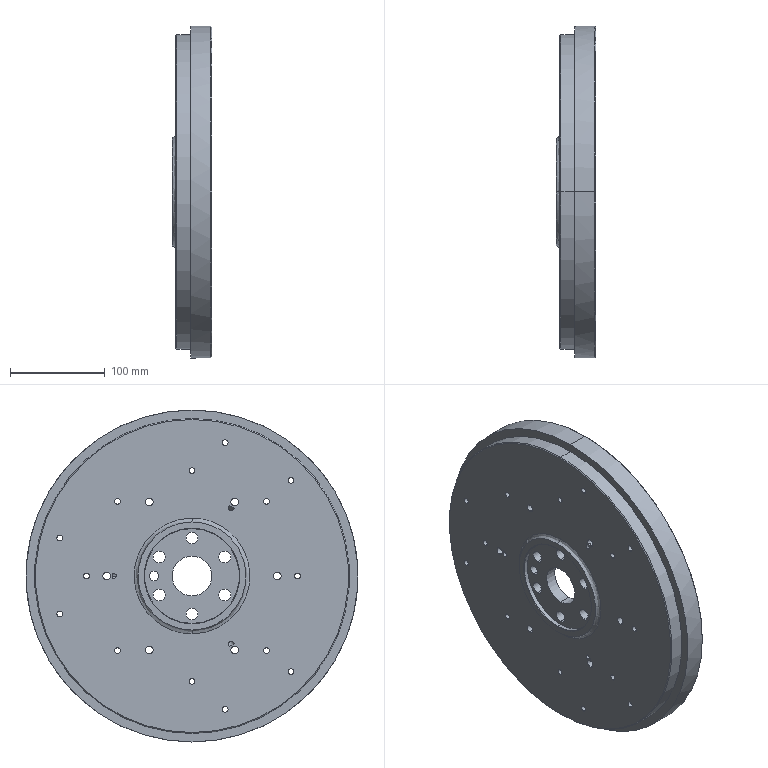Part | SolidWorks | features BaseBody 1 | 1 solid | 96 faces | box 42 x 350 x 350 mm | volume 2969350 mm3 | cylinder 72 | plane 10 | cone 8 | spline 6 | commonest cylinder face diameters 6 x34 8 x12 12.5 x12 10 x2 42 x2 100 x2